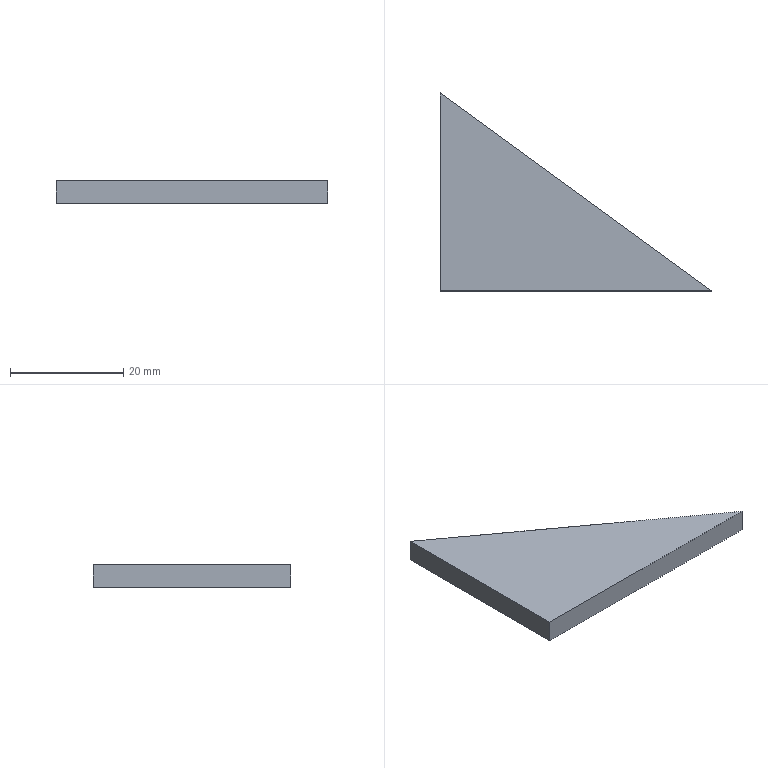Part | STEP file | E3-计量楼梯封Plate-125 | 1 solid | 5 faces | box 48 x 35 x 4 mm | volume 3360 mm3 | plane 5
STEP:
#1=CARTESIAN_POINT('',(0.,0.,0.));
#2=DIRECTION('',(0.,0.,1.));
#3=DIRECTION('',(1.,0.,0.));
#4=AXIS2_PLACEMENT_3D('',#1,#2,#3);
#5=CARTESIAN_POINT('',(0.,35.,0.));
#6=VERTEX_POINT('',#5);
#7=CARTESIAN_POINT('',(0.,0.,0.));
#8=VERTEX_POINT('',#7);
#9=CARTESIAN_POINT('',(0.,35.,0.));
#10=DIRECTION('',(0.,-1.,0.));
#11=VECTOR('',#10,1.);
#12=LINE('',#9,#11);
#13=CARTESIAN_POINT('',(0.,35.,-4.));
#14=DIRECTION('',(1.,0.,0.));
#15=DIRECTION('',(0.,1.,0.));
#16=AXIS2_PLACEMENT_3D('',#13,#14,#15);
#17=PLANE('',#16);
#18=CARTESIAN_POINT('',(0.,4.));
#19=DIRECTION('',(-1.,0.));
#20=VECTOR('',#19,1.);
#21=LINE('',#18,#20);
#22=(GEOMETRIC_REPRESENTATION_CONTEXT(2)PARAMETRIC_REPRESENTATION_CONTEXT()REPRESENTATION_CONTEXT('',''));
#23=DEFINITIONAL_REPRESENTATION('',(#21),#22);
#24=PCURVE('',#17,#23);
#25=CARTESIAN_POINT('',(0.,0.,0.));
#26=DIRECTION('',(0.,0.,-1.));
#27=DIRECTION('',(1.,0.,0.));
#28=AXIS2_PLACEMENT_3D('',#25,#26,#27);
#29=PLANE('',#28);
#30=CARTESIAN_POINT('',(0.,-35.));
#31=DIRECTION('',(0.,1.));
#32=VECTOR('',#31,1.);
#33=LINE('',#30,#32);
#34=(GEOMETRIC_REPRESENTATION_CONTEXT(2)PARAMETRIC_REPRESENTATION_CONTEXT()REPRESENTATION_CONTEXT('',''));
#35=DEFINITIONAL_REPRESENTATION('',(#33),#34);
#36=PCURVE('',#29,#35);
#37=SURFACE_CURVE('',#12,(#24,#36),.PCURVE_S1.);
#38=EDGE_CURVE('',#6,#8,#37,.T.);
#39=ORIENTED_EDGE('',*,*,#38,.F.);
#40=CARTESIAN_POINT('',(0.,35.,-4.));
#41=VERTEX_POINT('',#40);
#42=CARTESIAN_POINT('',(0.,35.,-4.));
#43=DIRECTION('',(0.,0.,1.));
#44=VECTOR('',#43,1.);
#45=LINE('',#42,#44);
#46=CARTESIAN_POINT('',(0.,0.));
#47=DIRECTION('',(0.,1.));
#48=VECTOR('',#47,1.);
#49=LINE('',#46,#48);
#50=(GEOMETRIC_REPRESENTATION_CONTEXT(2)PARAMETRIC_REPRESENTATION_CONTEXT()REPRESENTATION_CONTEXT('',''));
#51=DEFINITIONAL_REPRESENTATION('',(#49),#50);
#52=PCURVE('',#17,#51);
#53=CARTESIAN_POINT('',(48.,0.,-4.));
#54=DIRECTION('',(-0.5892,-0.808,0.));
#55=DIRECTION('',(0.808,-0.5892,0.));
#56=AXIS2_PLACEMENT_3D('',#53,#54,#55);
#57=PLANE('',#56);
#58=CARTESIAN_POINT('',(-59.405,0.));
#59=DIRECTION('',(0.,1.));
#60=VECTOR('',#59,1.);
#61=LINE('',#58,#60);
#62=(GEOMETRIC_REPRESENTATION_CONTEXT(2)PARAMETRIC_REPRESENTATION_CONTEXT()REPRESENTATION_CONTEXT('',''));
#63=DEFINITIONAL_REPRESENTATION('',(#61),#62);
#64=PCURVE('',#57,#63);
#65=SURFACE_CURVE('',#45,(#52,#64),.PCURVE_S1.);
#66=EDGE_CURVE('',#41,#6,#65,.T.);
#67=ORIENTED_EDGE('',*,*,#66,.F.);
#68=CARTESIAN_POINT('',(0.,0.,-4.));
#69=VERTEX_POINT('',#68);
#70=CARTESIAN_POINT('',(0.,35.,-4.));
#71=DIRECTION('',(0.,-1.,0.));
#72=VECTOR('',#71,1.);
#73=LINE('',#70,#72);
#74=CARTESIAN_POINT('',(0.,0.));
#75=DIRECTION('',(-1.,0.));
#76=VECTOR('',#75,1.);
#77=LINE('',#74,#76);
#78=(GEOMETRIC_REPRESENTATION_CONTEXT(2)PARAMETRIC_REPRESENTATION_CONTEXT()REPRESENTATION_CONTEXT('',''));
#79=DEFINITIONAL_REPRESENTATION('',(#77),#78);
#80=PCURVE('',#17,#79);
#81=CARTESIAN_POINT('',(0.,0.,-4.));
#82=DIRECTION('',(0.,0.,-1.));
#83=DIRECTION('',(1.,0.,0.));
#84=AXIS2_PLACEMENT_3D('',#81,#82,#83);
#85=PLANE('',#84);
#86=CARTESIAN_POINT('',(0.,-35.));
#87=DIRECTION('',(0.,1.));
#88=VECTOR('',#87,1.);
#89=LINE('',#86,#88);
#90=(GEOMETRIC_REPRESENTATION_CONTEXT(2)PARAMETRIC_REPRESENTATION_CONTEXT()REPRESENTATION_CONTEXT('',''));
#91=DEFINITIONAL_REPRESENTATION('',(#89),#90);
#92=PCURVE('',#85,#91);
#93=SURFACE_CURVE('',#73,(#80,#92),.PCURVE_S1.);
#94=EDGE_CURVE('',#41,#69,#93,.T.);
#95=ORIENTED_EDGE('',*,*,#94,.T.);
#96=CARTESIAN_POINT('',(0.,0.,-4.));
#97=DIRECTION('',(0.,0.,1.));
#98=VECTOR('',#97,1.);
#99=LINE('',#96,#98);
#100=CARTESIAN_POINT('',(-35.,0.));
#101=DIRECTION('',(0.,1.));
#102=VECTOR('',#101,1.);
#103=LINE('',#100,#102);
#104=(GEOMETRIC_REPRESENTATION_CONTEXT(2)PARAMETRIC_REPRESENTATION_CONTEXT()REPRESENTATION_CONTEXT('',''));
#105=DEFINITIONAL_REPRESENTATION('',(#103),#104);
#106=PCURVE('',#17,#105);
#107=CARTESIAN_POINT('',(0.,0.,-4.));
#108=DIRECTION('',(0.,1.,0.));
#109=DIRECTION('',(0.,0.,-1.));
#110=AXIS2_PLACEMENT_3D('',#107,#108,#109);
#111=PLANE('',#110);
#112=CARTESIAN_POINT('',(0.,0.));
#113=DIRECTION('',(-1.,0.));
#114=VECTOR('',#113,1.);
#115=LINE('',#112,#114);
#116=(GEOMETRIC_REPRESENTATION_CONTEXT(2)PARAMETRIC_REPRESENTATION_CONTEXT()REPRESENTATION_CONTEXT('',''));
#117=DEFINITIONAL_REPRESENTATION('',(#115),#116);
#118=PCURVE('',#111,#117);
#119=SURFACE_CURVE('',#99,(#106,#118),.PCURVE_S1.);
#120=EDGE_CURVE('',#69,#8,#119,.T.);
#121=ORIENTED_EDGE('',*,*,#120,.T.);
#122=EDGE_LOOP('',(#39,#67,#95,#121));
#123=FACE_BOUND('',#122,.T.);
#124=ADVANCED_FACE('',(#123),#17,.F.);
#125=CARTESIAN_POINT('',(48.,0.,0.));
#126=VERTEX_POINT('',#125);
#127=CARTESIAN_POINT('',(0.,0.,0.));
#128=DIRECTION('',(1.,0.,0.));
#129=VECTOR('',#128,1.);
#130=LINE('',#127,#129);
#131=CARTESIAN_POINT('',(-4.,0.));
#132=DIRECTION('',(0.,-1.));
#133=VECTOR('',#132,1.);
#134=LINE('',#131,#133);
#135=(GEOMETRIC_REPRESENTATION_CONTEXT(2)PARAMETRIC_REPRESENTATION_CONTEXT()REPRESENTATION_CONTEXT('',''));
#136=DEFINITIONAL_REPRESENTATION('',(#134),#135);
#137=PCURVE('',#111,#136);
#138=CARTESIAN_POINT('',(0.,0.));
#139=DIRECTION('',(1.,0.));
#140=VECTOR('',#139,1.);
#141=LINE('',#138,#140);
#142=(GEOMETRIC_REPRESENTATION_CONTEXT(2)PARAMETRIC_REPRESENTATION_CONTEXT()REPRESENTATION_CONTEXT('',''));
#143=DEFINITIONAL_REPRESENTATION('',(#141),#142);
#144=PCURVE('',#29,#143);
#145=SURFACE_CURVE('',#130,(#137,#144),.PCURVE_S1.);
#146=EDGE_CURVE('',#8,#126,#145,.T.);
#147=ORIENTED_EDGE('',*,*,#146,.F.);
#148=ORIENTED_EDGE('',*,*,#120,.F.);
#149=CARTESIAN_POINT('',(48.,0.,-4.));
#150=VERTEX_POINT('',#149);
#151=CARTESIAN_POINT('',(0.,0.,-4.));
#152=DIRECTION('',(1.,0.,0.));
#153=VECTOR('',#152,1.);
#154=LINE('',#151,#153);
#155=CARTESIAN_POINT('',(0.,0.));
#156=DIRECTION('',(0.,-1.));
#157=VECTOR('',#156,1.);
#158=LINE('',#155,#157);
#159=(GEOMETRIC_REPRESENTATION_CONTEXT(2)PARAMETRIC_REPRESENTATION_CONTEXT()REPRESENTATION_CONTEXT('',''));
#160=DEFINITIONAL_REPRESENTATION('',(#158),#159);
#161=PCURVE('',#111,#160);
#162=CARTESIAN_POINT('',(0.,0.));
#163=DIRECTION('',(1.,0.));
#164=VECTOR('',#163,1.);
#165=LINE('',#162,#164);
#166=(GEOMETRIC_REPRESENTATION_CONTEXT(2)PARAMETRIC_REPRESENTATION_CONTEXT()REPRESENTATION_CONTEXT('',''));
#167=DEFINITIONAL_REPRESENTATION('',(#165),#166);
#168=PCURVE('',#85,#167);
#169=SURFACE_CURVE('',#154,(#161,#168),.PCURVE_S1.);
#170=EDGE_CURVE('',#69,#150,#169,.T.);
#171=ORIENTED_EDGE('',*,*,#170,.T.);
#172=CARTESIAN_POINT('',(48.,0.,-4.));
#173=DIRECTION('',(0.,0.,1.));
#174=VECTOR('',#173,1.);
#175=LINE('',#172,#174);
#176=CARTESIAN_POINT('',(0.,-48.));
#177=DIRECTION('',(-1.,0.));
#178=VECTOR('',#177,1.);
#179=LINE('',#176,#178);
#180=(GEOMETRIC_REPRESENTATION_CONTEXT(2)PARAMETRIC_REPRESENTATION_CONTEXT()REPRESENTATION_CONTEXT('',''));
#181=DEFINITIONAL_REPRESENTATION('',(#179),#180);
#182=PCURVE('',#111,#181);
#183=CARTESIAN_POINT('',(0.,0.));
#184=DIRECTION('',(0.,1.));
#185=VECTOR('',#184,1.);
#186=LINE('',#183,#185);
#187=(GEOMETRIC_REPRESENTATION_CONTEXT(2)PARAMETRIC_REPRESENTATION_CONTEXT()REPRESENTATION_CONTEXT('',''));
#188=DEFINITIONAL_REPRESENTATION('',(#186),#187);
#189=PCURVE('',#57,#188);
#190=SURFACE_CURVE('',#175,(#182,#189),.PCURVE_S1.);
#191=EDGE_CURVE('',#150,#126,#190,.T.);
#192=ORIENTED_EDGE('',*,*,#191,.T.);
#193=EDGE_LOOP('',(#147,#148,#171,#192));
#194=FACE_BOUND('',#193,.T.);
#195=ADVANCED_FACE('',(#194),#111,.F.);
#196=CARTESIAN_POINT('',(48.,0.,0.));
#197=DIRECTION('',(-0.808,0.5892,0.));
#198=VECTOR('',#197,1.);
#199=LINE('',#196,#198);
#200=CARTESIAN_POINT('',(0.,4.));
#201=DIRECTION('',(-1.,0.));
#202=VECTOR('',#201,1.);
#203=LINE('',#200,#202);
#204=(GEOMETRIC_REPRESENTATION_CONTEXT(2)PARAMETRIC_REPRESENTATION_CONTEXT()REPRESENTATION_CONTEXT('',''));
#205=DEFINITIONAL_REPRESENTATION('',(#203),#204);
#206=PCURVE('',#57,#205);
#207=CARTESIAN_POINT('',(48.,0.));
#208=DIRECTION('',(-0.808,-0.5892));
#209=VECTOR('',#208,1.);
#210=LINE('',#207,#209);
#211=(GEOMETRIC_REPRESENTATION_CONTEXT(2)PARAMETRIC_REPRESENTATION_CONTEXT()REPRESENTATION_CONTEXT('',''));
#212=DEFINITIONAL_REPRESENTATION('',(#210),#211);
#213=PCURVE('',#29,#212);
#214=SURFACE_CURVE('',#199,(#206,#213),.PCURVE_S1.);
#215=EDGE_CURVE('',#126,#6,#214,.T.);
#216=ORIENTED_EDGE('',*,*,#215,.F.);
#217=ORIENTED_EDGE('',*,*,#191,.F.);
#218=CARTESIAN_POINT('',(48.,0.,-4.));
#219=DIRECTION('',(-0.808,0.5892,0.));
#220=VECTOR('',#219,1.);
#221=LINE('',#218,#220);
#222=CARTESIAN_POINT('',(0.,0.));
#223=DIRECTION('',(-1.,0.));
#224=VECTOR('',#223,1.);
#225=LINE('',#222,#224);
#226=(GEOMETRIC_REPRESENTATION_CONTEXT(2)PARAMETRIC_REPRESENTATION_CONTEXT()REPRESENTATION_CONTEXT('',''));
#227=DEFINITIONAL_REPRESENTATION('',(#225),#226);
#228=PCURVE('',#57,#227);
#229=CARTESIAN_POINT('',(48.,0.));
#230=DIRECTION('',(-0.808,-0.5892));
#231=VECTOR('',#230,1.);
#232=LINE('',#229,#231);
#233=(GEOMETRIC_REPRESENTATION_CONTEXT(2)PARAMETRIC_REPRESENTATION_CONTEXT()REPRESENTATION_CONTEXT('',''));
#234=DEFINITIONAL_REPRESENTATION('',(#232),#233);
#235=PCURVE('',#85,#234);
#236=SURFACE_CURVE('',#221,(#228,#235),.PCURVE_S1.);
#237=EDGE_CURVE('',#150,#41,#236,.T.);
#238=ORIENTED_EDGE('',*,*,#237,.T.);
#239=ORIENTED_EDGE('',*,*,#66,.T.);
#240=EDGE_LOOP('',(#216,#217,#238,#239));
#241=FACE_BOUND('',#240,.T.);
#242=ADVANCED_FACE('',(#241),#57,.F.);
#243=ORIENTED_EDGE('',*,*,#94,.F.);
#244=ORIENTED_EDGE('',*,*,#237,.F.);
#245=ORIENTED_EDGE('',*,*,#170,.F.);
#246=EDGE_LOOP('',(#243,#244,#245));
#247=FACE_BOUND('',#246,.T.);
#248=ADVANCED_FACE('',(#247),#85,.T.);
#249=ORIENTED_EDGE('',*,*,#38,.T.);
#250=ORIENTED_EDGE('',*,*,#146,.T.);
#251=ORIENTED_EDGE('',*,*,#215,.T.);
#252=EDGE_LOOP('',(#249,#250,#251));
#253=FACE_BOUND('',#252,.T.);
#254=ADVANCED_FACE('',(#253),#29,.F.);
#255=CLOSED_SHELL('',(#124,#195,#242,#248,#254));
#256=MANIFOLD_SOLID_BREP('',#255);
#257=(LENGTH_UNIT()NAMED_UNIT(*)SI_UNIT(.MILLI.,.METRE.));
#258=UNCERTAINTY_MEASURE_WITH_UNIT(LENGTH_MEASURE(0.0000001),#257,'','');
#259=(NAMED_UNIT(*)PLANE_ANGLE_UNIT()SI_UNIT($,.RADIAN.));
#260=(NAMED_UNIT(*)SI_UNIT($,.STERADIAN.)SOLID_ANGLE_UNIT());
#261=(GEOMETRIC_REPRESENTATION_CONTEXT(3)GLOBAL_UNCERTAINTY_ASSIGNED_CONTEXT((#258))GLOBAL_UNIT_ASSIGNED_CONTEXT((#257,#259,#260))REPRESENTATION_CONTEXT('',''));
#262=ADVANCED_BREP_SHAPE_REPRESENTATION('',(#4,#256),#261);